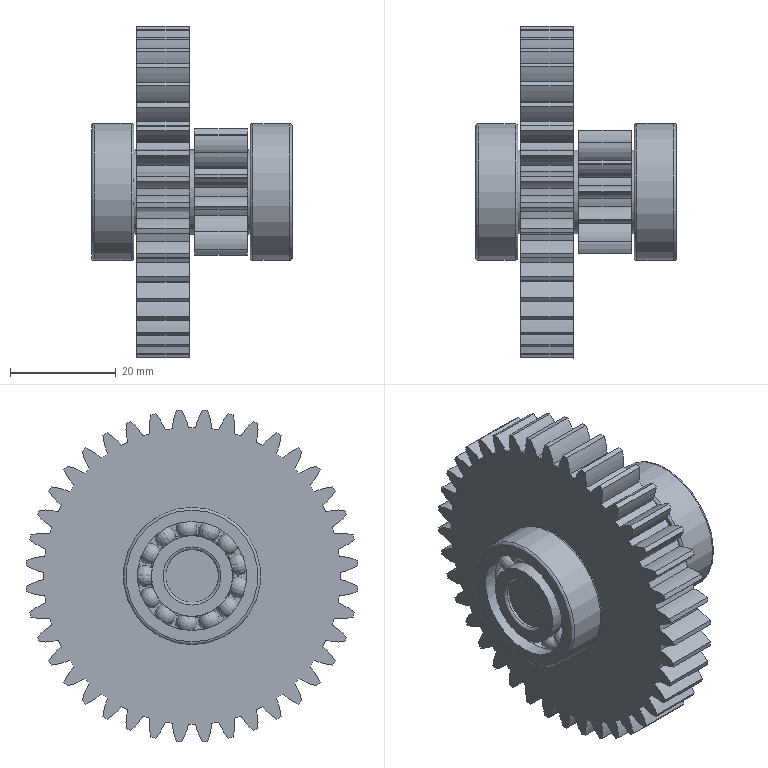Part | NX | features BREP 2 | 3 solids | 337 faces | box 38 x 62.873 x 62.873 mm | volume 38188 mm3 | cylinder 233 | torus 60 | sphere 26 | plane 16 | cone 2 | commonest cylinder face diameters 24 x94 56.248 x40 63 x40 8.391 x14 8.4 x14 17.248 x14